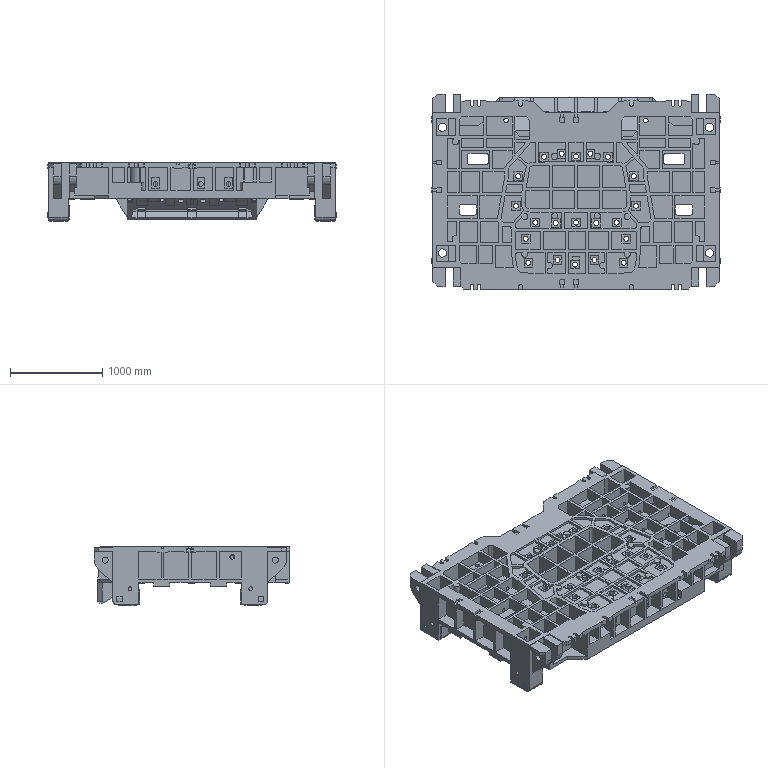Part | NX | features solid 2 | 1 solid | 2143 faces | box 3120 x 2120 x 635 mm | volume 784509833 mm3 | plane 1651 | cylinder 268 | spline 217 | cone 7 | commonest cylinder face diameters 40 x74 70 x29 55 x21 60 x18 36 x17 10 x14